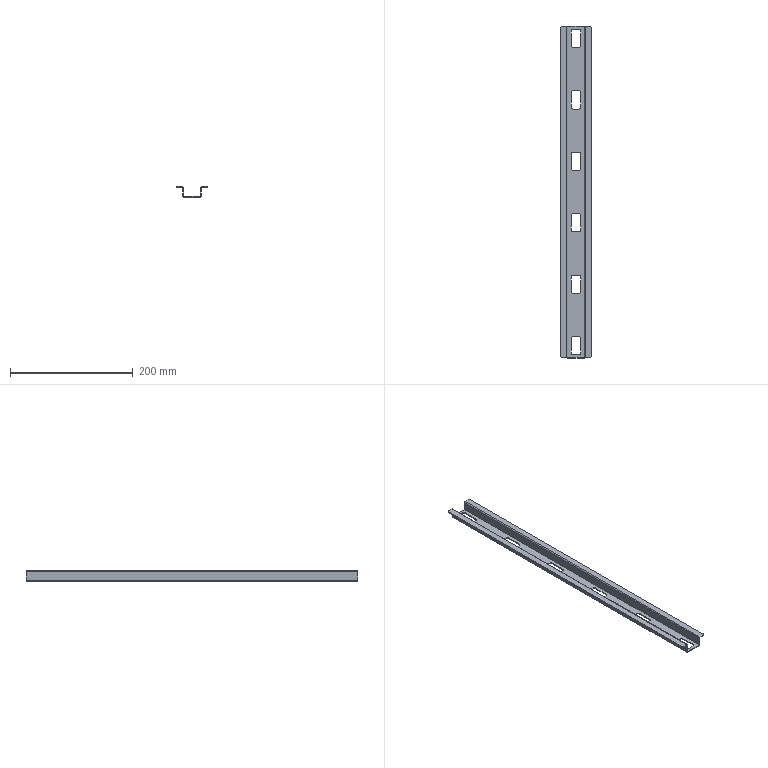Part | STEP file | HESS-408-70-15W-N-23-inner liner bottom plate reinforcing plate 1 | 1 solid | 74 faces | box 50 x 540 x 16.5 mm | volume 59626 mm3 | plane 38 | cylinder 36 | commonest cylinder face diameters 6 x28 0.2 x4 3.2 x4